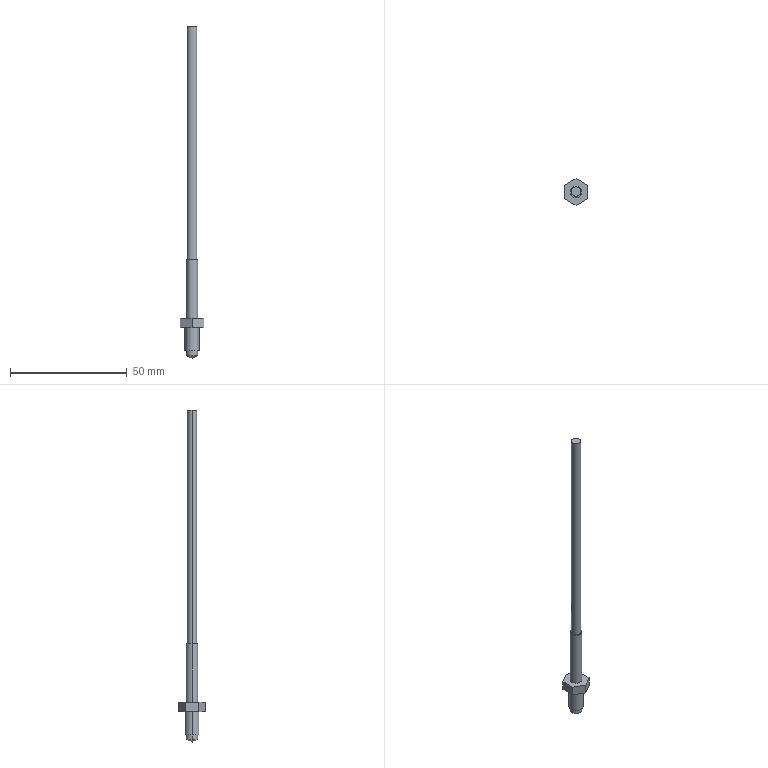Part | STEP file | 11-c-ssmt6-100011 | 1 solid | 21 faces | box 10 x 11.547 x 142 mm | volume 2422 mm3 | plane 11 | cylinder 8 | cone 2 | commonest cylinder face diameters 5 x4 4 x2 6 x2
STEP:
#1=CARTESIAN_POINT('',(69.774,-119.954,29.));
#2=VERTEX_POINT('',#1);
#3=CARTESIAN_POINT('',(65.774,-119.954,29.));
#4=VERTEX_POINT('',#3);
#5=CARTESIAN_POINT('',(67.774,-119.954,29.));
#6=DIRECTION('',(0.,0.,1.));
#7=DIRECTION('',(1.,0.,0.));
#8=AXIS2_PLACEMENT_3D('',#5,#6,#7);
#9=CIRCLE('',#8,2.);
#10=EDGE_CURVE('',#2,#4,#9,.T.);
#11=ORIENTED_EDGE('',*,*,#10,.T.);
#12=CARTESIAN_POINT('',(65.774,-119.954,129.));
#13=VERTEX_POINT('',#12);
#14=CARTESIAN_POINT('',(65.774,-119.954,29.));
#15=DIRECTION('',(0.,0.,1.));
#16=VECTOR('',#15,1000.);
#17=LINE('',#14,#16);
#18=EDGE_CURVE('',#4,#13,#17,.T.);
#19=ORIENTED_EDGE('',*,*,#18,.T.);
#20=CARTESIAN_POINT('',(69.774,-119.954,129.));
#21=VERTEX_POINT('',#20);
#22=CARTESIAN_POINT('',(67.774,-119.954,129.));
#23=DIRECTION('',(0.,0.,1.));
#24=DIRECTION('',(1.,0.,0.));
#25=AXIS2_PLACEMENT_3D('',#22,#23,#24);
#26=CIRCLE('',#25,2.);
#27=EDGE_CURVE('',#21,#13,#26,.T.);
#28=ORIENTED_EDGE('',*,*,#27,.F.);
#29=CARTESIAN_POINT('',(69.774,-119.954,29.));
#30=DIRECTION('',(0.,0.,1.));
#31=VECTOR('',#30,1000.);
#32=LINE('',#29,#31);
#33=EDGE_CURVE('',#2,#21,#32,.T.);
#34=ORIENTED_EDGE('',*,*,#33,.F.);
#35=EDGE_LOOP('',(#11,#19,#28,#34));
#36=FACE_OUTER_BOUND('',#35,.T.);
#37=CARTESIAN_POINT('',(67.774,-119.954,29.));
#38=DIRECTION('',(0.,0.,1.));
#39=DIRECTION('',(1.,0.,0.));
#40=AXIS2_PLACEMENT_3D('',#37,#38,#39);
#41=CYLINDRICAL_SURFACE('',#40,2.);
#42=ADVANCED_FACE('',(#36),#41,.T.);
#43=CARTESIAN_POINT('',(70.274,-119.954,4.));
#44=VERTEX_POINT('',#43);
#45=CARTESIAN_POINT('',(65.274,-119.954,4.));
#46=VERTEX_POINT('',#45);
#47=CARTESIAN_POINT('',(67.774,-119.954,4.));
#48=DIRECTION('',(0.,0.,1.));
#49=DIRECTION('',(1.,0.,0.));
#50=AXIS2_PLACEMENT_3D('',#47,#48,#49);
#51=CIRCLE('',#50,2.5);
#52=EDGE_CURVE('',#44,#46,#51,.T.);
#53=ORIENTED_EDGE('',*,*,#52,.T.);
#54=CARTESIAN_POINT('',(65.274,-119.954,29.));
#55=VERTEX_POINT('',#54);
#56=CARTESIAN_POINT('',(65.274,-119.954,4.));
#57=DIRECTION('',(0.,0.,1.));
#58=VECTOR('',#57,1000.);
#59=LINE('',#56,#58);
#60=EDGE_CURVE('',#46,#55,#59,.T.);
#61=ORIENTED_EDGE('',*,*,#60,.T.);
#62=CARTESIAN_POINT('',(70.274,-119.954,29.));
#63=VERTEX_POINT('',#62);
#64=CARTESIAN_POINT('',(67.774,-119.954,29.));
#65=DIRECTION('',(0.,0.,1.));
#66=DIRECTION('',(1.,0.,0.));
#67=AXIS2_PLACEMENT_3D('',#64,#65,#66);
#68=CIRCLE('',#67,2.5);
#69=EDGE_CURVE('',#63,#55,#68,.T.);
#70=ORIENTED_EDGE('',*,*,#69,.F.);
#71=CARTESIAN_POINT('',(70.274,-119.954,4.));
#72=DIRECTION('',(0.,0.,1.));
#73=VECTOR('',#72,1000.);
#74=LINE('',#71,#73);
#75=EDGE_CURVE('',#44,#63,#74,.T.);
#76=ORIENTED_EDGE('',*,*,#75,.F.);
#77=EDGE_LOOP('',(#53,#61,#70,#76));
#78=FACE_OUTER_BOUND('',#77,.T.);
#79=CARTESIAN_POINT('',(67.774,-119.954,4.));
#80=DIRECTION('',(0.,0.,1.));
#81=DIRECTION('',(1.,0.,0.));
#82=AXIS2_PLACEMENT_3D('',#79,#80,#81);
#83=CYLINDRICAL_SURFACE('',#82,2.5);
#84=ADVANCED_FACE('',(#78),#83,.T.);
#85=CARTESIAN_POINT('',(67.774,-119.954,-13.));
#86=VERTEX_POINT('',#85);
#87=CARTESIAN_POINT('',(70.274,-119.954,-12.));
#88=VERTEX_POINT('',#87);
#89=CARTESIAN_POINT('',(70.274,-119.954,-12.));
#90=DIRECTION('',(0.9285,0.,0.3714));
#91=VECTOR('',#90,1000.);
#92=LINE('',#89,#91);
#93=EDGE_CURVE('',#86,#88,#92,.T.);
#94=ORIENTED_EDGE('',*,*,#93,.F.);
#95=CARTESIAN_POINT('',(65.274,-119.954,-12.));
#96=VERTEX_POINT('',#95);
#97=CARTESIAN_POINT('',(65.274,-119.954,-12.));
#98=DIRECTION('',(-0.9285,0.,0.3714));
#99=VECTOR('',#98,1000.);
#100=LINE('',#97,#99);
#101=EDGE_CURVE('',#86,#96,#100,.T.);
#102=ORIENTED_EDGE('',*,*,#101,.T.);
#103=CARTESIAN_POINT('',(67.774,-119.954,-12.));
#104=DIRECTION('',(0.,0.,1.));
#105=DIRECTION('',(-1.,0.,0.));
#106=AXIS2_PLACEMENT_3D('',#103,#104,#105);
#107=CIRCLE('',#106,2.5);
#108=EDGE_CURVE('',#88,#96,#107,.T.);
#109=ORIENTED_EDGE('',*,*,#108,.F.);
#110=EDGE_LOOP('',(#94,#102,#109));
#111=FACE_OUTER_BOUND('',#110,.T.);
#112=CARTESIAN_POINT('',(67.774,-119.954,-12.));
#113=DIRECTION('',(0.,0.,1.));
#114=DIRECTION('',(1.,0.,0.));
#115=AXIS2_PLACEMENT_3D('',#112,#113,#114);
#116=CONICAL_SURFACE('',#115,2.5,1.19);
#117=ADVANCED_FACE('',(#111),#116,.T.);
#118=CARTESIAN_POINT('',(65.274,-119.954,-10.));
#119=VERTEX_POINT('',#118);
#120=CARTESIAN_POINT('',(70.274,-119.954,-10.));
#121=VERTEX_POINT('',#120);
#122=CARTESIAN_POINT('',(67.774,-119.954,-10.));
#123=DIRECTION('',(0.,0.,-1.));
#124=DIRECTION('',(-1.,0.,0.));
#125=AXIS2_PLACEMENT_3D('',#122,#123,#124);
#126=CIRCLE('',#125,2.5);
#127=EDGE_CURVE('',#119,#121,#126,.T.);
#128=ORIENTED_EDGE('',*,*,#127,.T.);
#129=CARTESIAN_POINT('',(70.274,-119.954,-10.));
#130=DIRECTION('',(0.,0.,-1.));
#131=VECTOR('',#130,1000.);
#132=LINE('',#129,#131);
#133=EDGE_CURVE('',#121,#88,#132,.T.);
#134=ORIENTED_EDGE('',*,*,#133,.T.);
#135=ORIENTED_EDGE('',*,*,#108,.T.);
#136=CARTESIAN_POINT('',(65.274,-119.954,-10.));
#137=DIRECTION('',(0.,0.,-1.));
#138=VECTOR('',#137,1000.);
#139=LINE('',#136,#138);
#140=EDGE_CURVE('',#119,#96,#139,.T.);
#141=ORIENTED_EDGE('',*,*,#140,.F.);
#142=EDGE_LOOP('',(#128,#134,#135,#141));
#143=FACE_OUTER_BOUND('',#142,.T.);
#144=CARTESIAN_POINT('',(67.774,-119.954,-10.));
#145=DIRECTION('',(0.,0.,-1.));
#146=DIRECTION('',(-1.,0.,0.));
#147=AXIS2_PLACEMENT_3D('',#144,#145,#146);
#148=CYLINDRICAL_SURFACE('',#147,2.5);
#149=ADVANCED_FACE('',(#143),#148,.T.);
#150=CARTESIAN_POINT('',(64.774,-119.954,0.));
#151=VERTEX_POINT('',#150);
#152=CARTESIAN_POINT('',(70.774,-119.954,0.));
#153=VERTEX_POINT('',#152);
#154=CARTESIAN_POINT('',(67.774,-119.954,0.));
#155=DIRECTION('',(0.,0.,-1.));
#156=DIRECTION('',(-1.,0.,0.));
#157=AXIS2_PLACEMENT_3D('',#154,#155,#156);
#158=CIRCLE('',#157,3.);
#159=EDGE_CURVE('',#151,#153,#158,.T.);
#160=ORIENTED_EDGE('',*,*,#159,.T.);
#161=CARTESIAN_POINT('',(70.774,-119.954,-10.));
#162=VERTEX_POINT('',#161);
#163=CARTESIAN_POINT('',(70.774,-119.954,0.));
#164=DIRECTION('',(0.,0.,-1.));
#165=VECTOR('',#164,1000.);
#166=LINE('',#163,#165);
#167=EDGE_CURVE('',#153,#162,#166,.T.);
#168=ORIENTED_EDGE('',*,*,#167,.T.);
#169=CARTESIAN_POINT('',(64.774,-119.954,-10.));
#170=VERTEX_POINT('',#169);
#171=CARTESIAN_POINT('',(67.774,-119.954,-10.));
#172=DIRECTION('',(0.,0.,-1.));
#173=DIRECTION('',(-1.,0.,0.));
#174=AXIS2_PLACEMENT_3D('',#171,#172,#173);
#175=CIRCLE('',#174,3.);
#176=EDGE_CURVE('',#170,#162,#175,.T.);
#177=ORIENTED_EDGE('',*,*,#176,.F.);
#178=CARTESIAN_POINT('',(64.774,-119.954,0.));
#179=DIRECTION('',(0.,0.,-1.));
#180=VECTOR('',#179,1000.);
#181=LINE('',#178,#180);
#182=EDGE_CURVE('',#151,#170,#181,.T.);
#183=ORIENTED_EDGE('',*,*,#182,.F.);
#184=EDGE_LOOP('',(#160,#168,#177,#183));
#185=FACE_OUTER_BOUND('',#184,.T.);
#186=CARTESIAN_POINT('',(67.774,-119.954,0.));
#187=DIRECTION('',(0.,0.,-1.));
#188=DIRECTION('',(-1.,0.,0.));
#189=AXIS2_PLACEMENT_3D('',#186,#187,#188);
#190=CYLINDRICAL_SURFACE('',#189,3.);
#191=ADVANCED_FACE('',(#185),#190,.T.);
#192=CARTESIAN_POINT('',(72.774,-122.841,0.));
#193=VERTEX_POINT('',#192);
#194=CARTESIAN_POINT('',(67.774,-125.728,0.));
#195=VERTEX_POINT('',#194);
#196=CARTESIAN_POINT('',(72.774,-122.841,0.));
#197=DIRECTION('',(-0.866,-0.5,0.));
#198=VECTOR('',#197,1000.);
#199=LINE('',#196,#198);
#200=EDGE_CURVE('',#193,#195,#199,.T.);
#201=ORIENTED_EDGE('',*,*,#200,.F.);
#202=CARTESIAN_POINT('',(72.774,-122.841,4.));
#203=VERTEX_POINT('',#202);
#204=CARTESIAN_POINT('',(72.774,-122.841,4.));
#205=DIRECTION('',(0.,0.,-1.));
#206=VECTOR('',#205,1000.);
#207=LINE('',#204,#206);
#208=EDGE_CURVE('',#203,#193,#207,.T.);
#209=ORIENTED_EDGE('',*,*,#208,.F.);
#210=CARTESIAN_POINT('',(67.774,-125.728,4.));
#211=VERTEX_POINT('',#210);
#212=CARTESIAN_POINT('',(72.774,-122.841,4.));
#213=DIRECTION('',(-0.866,-0.5,0.));
#214=VECTOR('',#213,1000.);
#215=LINE('',#212,#214);
#216=EDGE_CURVE('',#203,#211,#215,.T.);
#217=ORIENTED_EDGE('',*,*,#216,.T.);
#218=CARTESIAN_POINT('',(67.774,-125.728,4.));
#219=DIRECTION('',(0.,0.,-1.));
#220=VECTOR('',#219,1000.);
#221=LINE('',#218,#220);
#222=EDGE_CURVE('',#211,#195,#221,.T.);
#223=ORIENTED_EDGE('',*,*,#222,.T.);
#224=EDGE_LOOP('',(#201,#209,#217,#223));
#225=FACE_OUTER_BOUND('',#224,.T.);
#226=CARTESIAN_POINT('',(72.774,-122.841,4.));
#227=DIRECTION('',(0.5,-0.866,0.));
#228=DIRECTION('',(0.866,0.5,0.));
#229=AXIS2_PLACEMENT_3D('',#226,#227,#228);
#230=PLANE('',#229);
#231=ADVANCED_FACE('',(#225),#230,.T.);
#232=CARTESIAN_POINT('',(62.774,-122.841,0.));
#233=VERTEX_POINT('',#232);
#234=CARTESIAN_POINT('',(67.774,-125.728,0.));
#235=DIRECTION('',(-0.866,0.5,0.));
#236=VECTOR('',#235,1000.);
#237=LINE('',#234,#236);
#238=EDGE_CURVE('',#195,#233,#237,.T.);
#239=ORIENTED_EDGE('',*,*,#238,.F.);
#240=ORIENTED_EDGE('',*,*,#222,.F.);
#241=CARTESIAN_POINT('',(62.774,-122.841,4.));
#242=VERTEX_POINT('',#241);
#243=CARTESIAN_POINT('',(67.774,-125.728,4.));
#244=DIRECTION('',(-0.866,0.5,0.));
#245=VECTOR('',#244,1000.);
#246=LINE('',#243,#245);
#247=EDGE_CURVE('',#211,#242,#246,.T.);
#248=ORIENTED_EDGE('',*,*,#247,.T.);
#249=CARTESIAN_POINT('',(62.774,-122.841,4.));
#250=DIRECTION('',(0.,0.,-1.));
#251=VECTOR('',#250,1000.);
#252=LINE('',#249,#251);
#253=EDGE_CURVE('',#242,#233,#252,.T.);
#254=ORIENTED_EDGE('',*,*,#253,.T.);
#255=EDGE_LOOP('',(#239,#240,#248,#254));
#256=FACE_OUTER_BOUND('',#255,.T.);
#257=CARTESIAN_POINT('',(67.774,-125.728,4.));
#258=DIRECTION('',(-0.5,-0.866,0.));
#259=DIRECTION('',(0.866,-0.5,0.));
#260=AXIS2_PLACEMENT_3D('',#257,#258,#259);
#261=PLANE('',#260);
#262=ADVANCED_FACE('',(#256),#261,.T.);
#263=CARTESIAN_POINT('',(62.774,-117.067,0.));
#264=VERTEX_POINT('',#263);
#265=CARTESIAN_POINT('',(62.774,-122.841,0.));
#266=DIRECTION('',(0.,1.,0.));
#267=VECTOR('',#266,1000.);
#268=LINE('',#265,#267);
#269=EDGE_CURVE('',#233,#264,#268,.T.);
#270=ORIENTED_EDGE('',*,*,#269,.F.);
#271=ORIENTED_EDGE('',*,*,#253,.F.);
#272=CARTESIAN_POINT('',(62.774,-117.067,4.));
#273=VERTEX_POINT('',#272);
#274=CARTESIAN_POINT('',(62.774,-122.841,4.));
#275=DIRECTION('',(0.,1.,0.));
#276=VECTOR('',#275,1000.);
#277=LINE('',#274,#276);
#278=EDGE_CURVE('',#242,#273,#277,.T.);
#279=ORIENTED_EDGE('',*,*,#278,.T.);
#280=CARTESIAN_POINT('',(62.774,-117.067,4.));
#281=DIRECTION('',(0.,0.,-1.));
#282=VECTOR('',#281,1000.);
#283=LINE('',#280,#282);
#284=EDGE_CURVE('',#273,#264,#283,.T.);
#285=ORIENTED_EDGE('',*,*,#284,.T.);
#286=EDGE_LOOP('',(#270,#271,#279,#285));
#287=FACE_OUTER_BOUND('',#286,.T.);
#288=CARTESIAN_POINT('',(62.774,-122.841,4.));
#289=DIRECTION('',(-1.,0.,0.));
#290=DIRECTION('',(0.,-1.,0.));
#291=AXIS2_PLACEMENT_3D('',#288,#289,#290);
#292=PLANE('',#291);
#293=ADVANCED_FACE('',(#287),#292,.T.);
#294=CARTESIAN_POINT('',(67.774,-114.181,0.));
#295=VERTEX_POINT('',#294);
#296=CARTESIAN_POINT('',(62.774,-117.067,0.));
#297=DIRECTION('',(0.866,0.5,0.));
#298=VECTOR('',#297,1000.);
#299=LINE('',#296,#298);
#300=EDGE_CURVE('',#264,#295,#299,.T.);
#301=ORIENTED_EDGE('',*,*,#300,.F.);
#302=ORIENTED_EDGE('',*,*,#284,.F.);
#303=CARTESIAN_POINT('',(67.774,-114.181,4.));
#304=VERTEX_POINT('',#303);
#305=CARTESIAN_POINT('',(62.774,-117.067,4.));
#306=DIRECTION('',(0.866,0.5,0.));
#307=VECTOR('',#306,1000.);
#308=LINE('',#305,#307);
#309=EDGE_CURVE('',#273,#304,#308,.T.);
#310=ORIENTED_EDGE('',*,*,#309,.T.);
#311=CARTESIAN_POINT('',(67.774,-114.181,4.));
#312=DIRECTION('',(0.,0.,-1.));
#313=VECTOR('',#312,1000.);
#314=LINE('',#311,#313);
#315=EDGE_CURVE('',#304,#295,#314,.T.);
#316=ORIENTED_EDGE('',*,*,#315,.T.);
#317=EDGE_LOOP('',(#301,#302,#310,#316));
#318=FACE_OUTER_BOUND('',#317,.T.);
#319=CARTESIAN_POINT('',(62.774,-117.067,4.));
#320=DIRECTION('',(-0.5,0.866,0.));
#321=DIRECTION('',(-0.866,-0.5,0.));
#322=AXIS2_PLACEMENT_3D('',#319,#320,#321);
#323=PLANE('',#322);
#324=ADVANCED_FACE('',(#318),#323,.T.);
#325=CARTESIAN_POINT('',(72.774,-117.067,0.));
#326=VERTEX_POINT('',#325);
#327=CARTESIAN_POINT('',(67.774,-114.181,0.));
#328=DIRECTION('',(0.866,-0.5,0.));
#329=VECTOR('',#328,1000.);
#330=LINE('',#327,#329);
#331=EDGE_CURVE('',#295,#326,#330,.T.);
#332=ORIENTED_EDGE('',*,*,#331,.F.);
#333=ORIENTED_EDGE('',*,*,#315,.F.);
#334=CARTESIAN_POINT('',(72.774,-117.067,4.));
#335=VERTEX_POINT('',#334);
#336=CARTESIAN_POINT('',(67.774,-114.181,4.));
#337=DIRECTION('',(0.866,-0.5,0.));
#338=VECTOR('',#337,1000.);
#339=LINE('',#336,#338);
#340=EDGE_CURVE('',#304,#335,#339,.T.);
#341=ORIENTED_EDGE('',*,*,#340,.T.);
#342=CARTESIAN_POINT('',(72.774,-117.067,4.));
#343=DIRECTION('',(0.,0.,-1.));
#344=VECTOR('',#343,1000.);
#345=LINE('',#342,#344);
#346=EDGE_CURVE('',#335,#326,#345,.T.);
#347=ORIENTED_EDGE('',*,*,#346,.T.);
#348=EDGE_LOOP('',(#332,#333,#341,#347));
#349=FACE_OUTER_BOUND('',#348,.T.);
#350=CARTESIAN_POINT('',(67.774,-114.181,4.));
#351=DIRECTION('',(0.5,0.866,0.));
#352=DIRECTION('',(-0.866,0.5,0.));
#353=AXIS2_PLACEMENT_3D('',#350,#351,#352);
#354=PLANE('',#353);
#355=ADVANCED_FACE('',(#349),#354,.T.);
#356=CARTESIAN_POINT('',(72.774,-117.067,0.));
#357=DIRECTION('',(0.,-1.,0.));
#358=VECTOR('',#357,1000.);
#359=LINE('',#356,#358);
#360=EDGE_CURVE('',#326,#193,#359,.T.);
#361=ORIENTED_EDGE('',*,*,#360,.F.);
#362=ORIENTED_EDGE('',*,*,#346,.F.);
#363=CARTESIAN_POINT('',(72.774,-117.067,4.));
#364=DIRECTION('',(0.,-1.,0.));
#365=VECTOR('',#364,1000.);
#366=LINE('',#363,#365);
#367=EDGE_CURVE('',#335,#203,#366,.T.);
#368=ORIENTED_EDGE('',*,*,#367,.T.);
#369=ORIENTED_EDGE('',*,*,#208,.T.);
#370=EDGE_LOOP('',(#361,#362,#368,#369));
#371=FACE_OUTER_BOUND('',#370,.T.);
#372=CARTESIAN_POINT('',(72.774,-117.067,4.));
#373=DIRECTION('',(1.,0.,0.));
#374=DIRECTION('',(0.,0.,-1.));
#375=AXIS2_PLACEMENT_3D('',#372,#373,#374);
#376=PLANE('',#375);
#377=ADVANCED_FACE('',(#371),#376,.T.);
#378=ORIENTED_EDGE('',*,*,#52,.F.);
#379=CARTESIAN_POINT('',(67.774,-119.954,4.));
#380=DIRECTION('',(0.,0.,1.));
#381=DIRECTION('',(1.,0.,0.));
#382=AXIS2_PLACEMENT_3D('',#379,#380,#381);
#383=CIRCLE('',#382,2.5);
#384=EDGE_CURVE('',#46,#44,#383,.T.);
#385=ORIENTED_EDGE('',*,*,#384,.F.);
#386=EDGE_LOOP('',(#378,#385));
#387=FACE_BOUND('',#386,.T.);
#388=ORIENTED_EDGE('',*,*,#216,.F.);
#389=ORIENTED_EDGE('',*,*,#367,.F.);
#390=ORIENTED_EDGE('',*,*,#340,.F.);
#391=ORIENTED_EDGE('',*,*,#309,.F.);
#392=ORIENTED_EDGE('',*,*,#278,.F.);
#393=ORIENTED_EDGE('',*,*,#247,.F.);
#394=EDGE_LOOP('',(#388,#389,#390,#391,#392,#393));
#395=FACE_OUTER_BOUND('',#394,.T.);
#396=CARTESIAN_POINT('',(62.774,-128.614,4.));
#397=DIRECTION('',(0.,0.,-1.));
#398=DIRECTION('',(-1.,0.,0.));
#399=AXIS2_PLACEMENT_3D('',#396,#397,#398);
#400=PLANE('',#399);
#401=ADVANCED_FACE('',(#387,#395),#400,.F.);
#402=ORIENTED_EDGE('',*,*,#159,.F.);
#403=CARTESIAN_POINT('',(67.774,-119.954,0.));
#404=DIRECTION('',(0.,0.,-1.));
#405=DIRECTION('',(-1.,0.,0.));
#406=AXIS2_PLACEMENT_3D('',#403,#404,#405);
#407=CIRCLE('',#406,3.);
#408=EDGE_CURVE('',#153,#151,#407,.T.);
#409=ORIENTED_EDGE('',*,*,#408,.F.);
#410=EDGE_LOOP('',(#402,#409));
#411=FACE_BOUND('',#410,.T.);
#412=ORIENTED_EDGE('',*,*,#200,.T.);
#413=ORIENTED_EDGE('',*,*,#238,.T.);
#414=ORIENTED_EDGE('',*,*,#269,.T.);
#415=ORIENTED_EDGE('',*,*,#300,.T.);
#416=ORIENTED_EDGE('',*,*,#331,.T.);
#417=ORIENTED_EDGE('',*,*,#360,.T.);
#418=EDGE_LOOP('',(#412,#413,#414,#415,#416,#417));
#419=FACE_OUTER_BOUND('',#418,.T.);
#420=CARTESIAN_POINT('',(62.774,-128.614,0.));
#421=DIRECTION('',(0.,0.,-1.));
#422=DIRECTION('',(-1.,0.,0.));
#423=AXIS2_PLACEMENT_3D('',#420,#421,#422);
#424=PLANE('',#423);
#425=ADVANCED_FACE('',(#411,#419),#424,.T.);
#426=ORIENTED_EDGE('',*,*,#127,.F.);
#427=CARTESIAN_POINT('',(67.774,-119.954,-10.));
#428=DIRECTION('',(0.,0.,-1.));
#429=DIRECTION('',(-1.,0.,0.));
#430=AXIS2_PLACEMENT_3D('',#427,#428,#429);
#431=CIRCLE('',#430,2.5);
#432=EDGE_CURVE('',#121,#119,#431,.T.);
#433=ORIENTED_EDGE('',*,*,#432,.F.);
#434=EDGE_LOOP('',(#426,#433));
#435=FACE_BOUND('',#434,.T.);
#436=ORIENTED_EDGE('',*,*,#176,.T.);
#437=CARTESIAN_POINT('',(67.774,-119.954,-10.));
#438=DIRECTION('',(0.,0.,-1.));
#439=DIRECTION('',(-1.,0.,0.));
#440=AXIS2_PLACEMENT_3D('',#437,#438,#439);
#441=CIRCLE('',#440,3.);
#442=EDGE_CURVE('',#162,#170,#441,.T.);
#443=ORIENTED_EDGE('',*,*,#442,.T.);
#444=EDGE_LOOP('',(#436,#443));
#445=FACE_OUTER_BOUND('',#444,.T.);
#446=CARTESIAN_POINT('',(67.774,-119.954,-10.));
#447=DIRECTION('',(0.,0.,-1.));
#448=DIRECTION('',(-1.,0.,0.));
#449=AXIS2_PLACEMENT_3D('',#446,#447,#448);
#450=PLANE('',#449);
#451=ADVANCED_FACE('',(#435,#445),#450,.T.);
#452=ORIENTED_EDGE('',*,*,#167,.F.);
#453=ORIENTED_EDGE('',*,*,#408,.T.);
#454=ORIENTED_EDGE('',*,*,#182,.T.);
#455=ORIENTED_EDGE('',*,*,#442,.F.);
#456=EDGE_LOOP('',(#452,#453,#454,#455));
#457=FACE_OUTER_BOUND('',#456,.T.);
#458=CARTESIAN_POINT('',(67.774,-119.954,0.));
#459=DIRECTION('',(0.,0.,-1.));
#460=DIRECTION('',(-1.,0.,0.));
#461=AXIS2_PLACEMENT_3D('',#458,#459,#460);
#462=CYLINDRICAL_SURFACE('',#461,3.);
#463=ADVANCED_FACE('',(#457),#462,.T.);
#464=ORIENTED_EDGE('',*,*,#133,.F.);
#465=ORIENTED_EDGE('',*,*,#432,.T.);
#466=ORIENTED_EDGE('',*,*,#140,.T.);
#467=CARTESIAN_POINT('',(67.774,-119.954,-12.));
#468=DIRECTION('',(0.,0.,1.));
#469=DIRECTION('',(-1.,0.,0.));
#470=AXIS2_PLACEMENT_3D('',#467,#468,#469);
#471=CIRCLE('',#470,2.5);
#472=EDGE_CURVE('',#96,#88,#471,.T.);
#473=ORIENTED_EDGE('',*,*,#472,.T.);
#474=EDGE_LOOP('',(#464,#465,#466,#473));
#475=FACE_OUTER_BOUND('',#474,.T.);
#476=CARTESIAN_POINT('',(67.774,-119.954,-10.));
#477=DIRECTION('',(0.,0.,-1.));
#478=DIRECTION('',(-1.,0.,0.));
#479=AXIS2_PLACEMENT_3D('',#476,#477,#478);
#480=CYLINDRICAL_SURFACE('',#479,2.5);
#481=ADVANCED_FACE('',(#475),#480,.T.);
#482=ORIENTED_EDGE('',*,*,#101,.F.);
#483=ORIENTED_EDGE('',*,*,#93,.T.);
#484=ORIENTED_EDGE('',*,*,#472,.F.);
#485=EDGE_LOOP('',(#482,#483,#484));
#486=FACE_OUTER_BOUND('',#485,.T.);
#487=CARTESIAN_POINT('',(67.774,-119.954,-12.));
#488=DIRECTION('',(0.,0.,1.));
#489=DIRECTION('',(1.,0.,0.));
#490=AXIS2_PLACEMENT_3D('',#487,#488,#489);
#491=CONICAL_SURFACE('',#490,2.5,1.19);
#492=ADVANCED_FACE('',(#486),#491,.T.);
#493=ORIENTED_EDGE('',*,*,#10,.F.);
#494=CARTESIAN_POINT('',(67.774,-119.954,29.));
#495=DIRECTION('',(0.,0.,1.));
#496=DIRECTION('',(1.,0.,0.));
#497=AXIS2_PLACEMENT_3D('',#494,#495,#496);
#498=CIRCLE('',#497,2.);
#499=EDGE_CURVE('',#4,#2,#498,.T.);
#500=ORIENTED_EDGE('',*,*,#499,.F.);
#501=EDGE_LOOP('',(#493,#500));
#502=FACE_BOUND('',#501,.T.);
#503=ORIENTED_EDGE('',*,*,#69,.T.);
#504=CARTESIAN_POINT('',(67.774,-119.954,29.));
#505=DIRECTION('',(0.,0.,1.));
#506=DIRECTION('',(1.,0.,0.));
#507=AXIS2_PLACEMENT_3D('',#504,#505,#506);
#508=CIRCLE('',#507,2.5);
#509=EDGE_CURVE('',#55,#63,#508,.T.);
#510=ORIENTED_EDGE('',*,*,#509,.T.);
#511=EDGE_LOOP('',(#503,#510));
#512=FACE_OUTER_BOUND('',#511,.T.);
#513=CARTESIAN_POINT('',(67.774,-119.954,29.));
#514=DIRECTION('',(0.,0.,1.));
#515=DIRECTION('',(1.,0.,0.));
#516=AXIS2_PLACEMENT_3D('',#513,#514,#515);
#517=PLANE('',#516);
#518=ADVANCED_FACE('',(#502,#512),#517,.T.);
#519=ORIENTED_EDGE('',*,*,#60,.F.);
#520=ORIENTED_EDGE('',*,*,#384,.T.);
#521=ORIENTED_EDGE('',*,*,#75,.T.);
#522=ORIENTED_EDGE('',*,*,#509,.F.);
#523=EDGE_LOOP('',(#519,#520,#521,#522));
#524=FACE_OUTER_BOUND('',#523,.T.);
#525=CARTESIAN_POINT('',(67.774,-119.954,4.));
#526=DIRECTION('',(0.,0.,1.));
#527=DIRECTION('',(1.,0.,0.));
#528=AXIS2_PLACEMENT_3D('',#525,#526,#527);
#529=CYLINDRICAL_SURFACE('',#528,2.5);
#530=ADVANCED_FACE('',(#524),#529,.T.);
#531=ORIENTED_EDGE('',*,*,#27,.T.);
#532=CARTESIAN_POINT('',(67.774,-119.954,129.));
#533=DIRECTION('',(0.,0.,1.));
#534=DIRECTION('',(1.,0.,0.));
#535=AXIS2_PLACEMENT_3D('',#532,#533,#534);
#536=CIRCLE('',#535,2.);
#537=EDGE_CURVE('',#13,#21,#536,.T.);
#538=ORIENTED_EDGE('',*,*,#537,.T.);
#539=EDGE_LOOP('',(#531,#538));
#540=FACE_OUTER_BOUND('',#539,.T.);
#541=CARTESIAN_POINT('',(67.774,-119.954,129.));
#542=DIRECTION('',(0.,0.,1.));
#543=DIRECTION('',(1.,0.,0.));
#544=AXIS2_PLACEMENT_3D('',#541,#542,#543);
#545=PLANE('',#544);
#546=ADVANCED_FACE('',(#540),#545,.T.);
#547=ORIENTED_EDGE('',*,*,#18,.F.);
#548=ORIENTED_EDGE('',*,*,#499,.T.);
#549=ORIENTED_EDGE('',*,*,#33,.T.);
#550=ORIENTED_EDGE('',*,*,#537,.F.);
#551=EDGE_LOOP('',(#547,#548,#549,#550));
#552=FACE_OUTER_BOUND('',#551,.T.);
#553=CARTESIAN_POINT('',(67.774,-119.954,29.));
#554=DIRECTION('',(0.,0.,1.));
#555=DIRECTION('',(1.,0.,0.));
#556=AXIS2_PLACEMENT_3D('',#553,#554,#555);
#557=CYLINDRICAL_SURFACE('',#556,2.);
#558=ADVANCED_FACE('',(#552),#557,.T.);
#559=CLOSED_SHELL('',(#42,#84,#117,#149,#191,#231,#262,#293,#324,#355,#377,#401,#425,#451,#463,#481,#492,#518,#530,#546,#558));
#560=MANIFOLD_SOLID_BREP('',#559);
#561=CARTESIAN_POINT('',(0.,0.,0.));
#562=DIRECTION('',(0.,0.,1.));
#563=DIRECTION('',(1.,0.,0.));
#564=AXIS2_PLACEMENT_3D('',#561,#562,#563);
#565=(LENGTH_UNIT()NAMED_UNIT(*)SI_UNIT(.MILLI.,.METRE.));
#566=UNCERTAINTY_MEASURE_WITH_UNIT(LENGTH_MEASURE(0.00001),#565,'','');
#567=(NAMED_UNIT(*)PLANE_ANGLE_UNIT()SI_UNIT($,.RADIAN.));
#568=(NAMED_UNIT(*)SI_UNIT($,.STERADIAN.)SOLID_ANGLE_UNIT());
#569=(GEOMETRIC_REPRESENTATION_CONTEXT(3)GLOBAL_UNCERTAINTY_ASSIGNED_CONTEXT((#566))GLOBAL_UNIT_ASSIGNED_CONTEXT((#565,#567,#568))REPRESENTATION_CONTEXT('',''));
#570=ADVANCED_BREP_SHAPE_REPRESENTATION('',(#560,#564),#569);